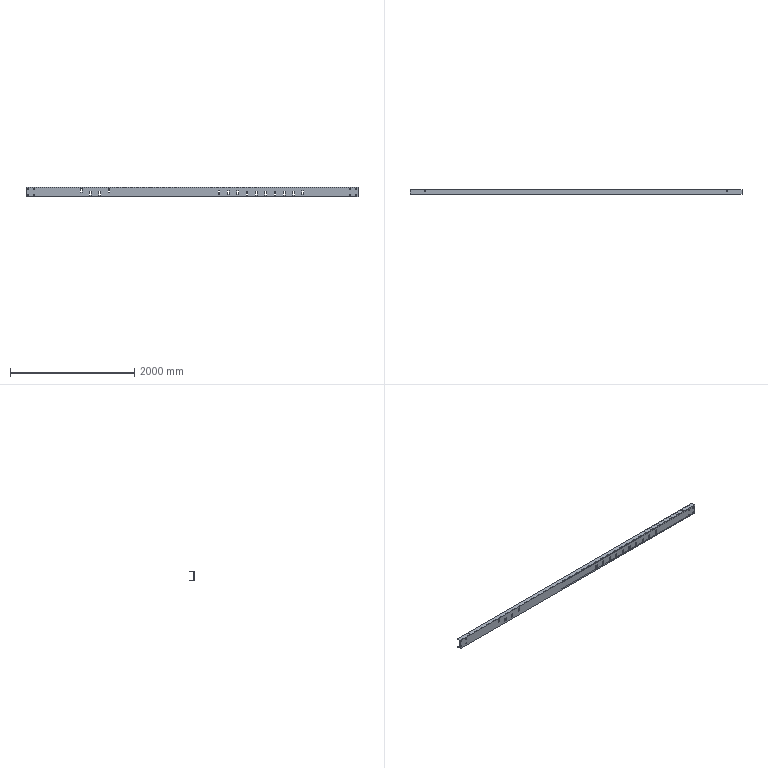Part | STEP file | 05-Left main beam 1_default<machining> | 1 solid | 90 faces | box 5344 x 65 x 160 mm | volume 13076241 mm3 | plane 66 | cylinder 24 | commonest cylinder face diameters 18 x16 10 x6 20 x2